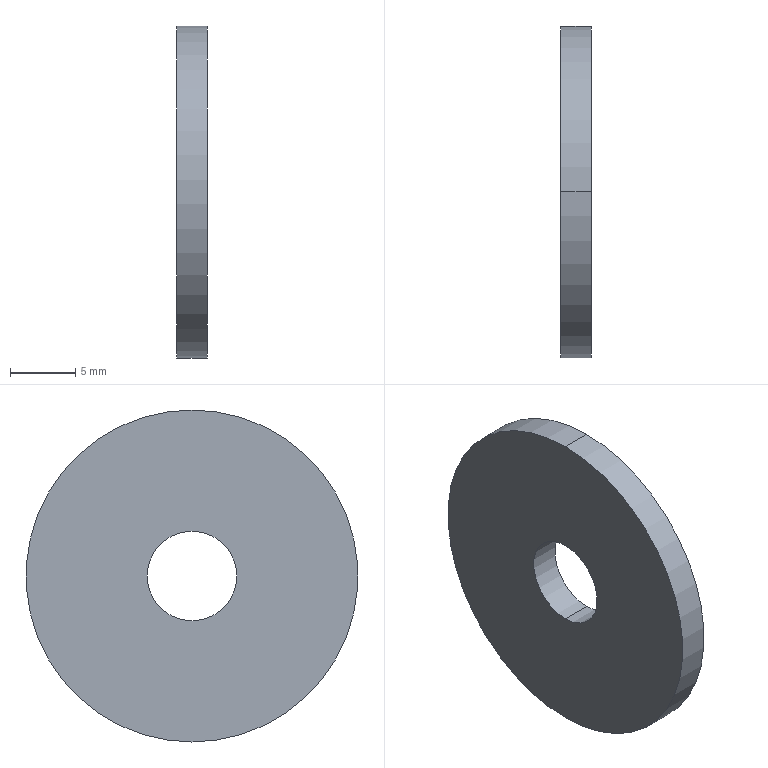Part | STEP file | flat washer wide_am_B18.22M - Plain washer, 6 mm, wide | 1 solid | 6 faces | box 2.3 x 25.4 x 25.4 mm | volume 1080 mm3 | cylinder 4 | plane 2 | commonest cylinder face diameters 6.87 x2 25.4 x2
STEP:
#1=CARTESIAN_POINT('',(0.,0.,0.));
#2=DIRECTION('',(0.,0.,1.));
#3=DIRECTION('',(1.,0.,0.));
#4=AXIS2_PLACEMENT_3D('',#1,#2,#3);
#5=CARTESIAN_POINT('',(0.,0.,12.7));
#6=VERTEX_POINT('',#5);
#7=CARTESIAN_POINT('',(0.,0.,-12.7));
#8=VERTEX_POINT('',#7);
#9=CARTESIAN_POINT('',(0.,0.,0.));
#10=DIRECTION('',(-1.,0.,0.));
#11=DIRECTION('',(0.,0.,1.));
#12=AXIS2_PLACEMENT_3D('',#9,#10,#11);
#13=CIRCLE('',#12,12.7);
#14=CARTESIAN_POINT('',(-34.925,0.,0.));
#15=DIRECTION('',(-1.,0.,0.));
#16=DIRECTION('',(0.,0.,1.));
#17=AXIS2_PLACEMENT_3D('',#14,#15,#16);
#18=CYLINDRICAL_SURFACE('',#17,12.7);
#19=CARTESIAN_POINT('',(0.,-34.925));
#20=DIRECTION('',(1.,0.));
#21=VECTOR('',#20,1.);
#22=LINE('',#19,#21);
#23=(GEOMETRIC_REPRESENTATION_CONTEXT(2)PARAMETRIC_REPRESENTATION_CONTEXT()REPRESENTATION_CONTEXT('',''));
#24=DEFINITIONAL_REPRESENTATION('',(#22),#23);
#25=PCURVE('',#18,#24);
#26=CARTESIAN_POINT('',(0.,3.435,0.));
#27=DIRECTION('',(-1.,0.,0.));
#28=DIRECTION('',(0.,0.,1.));
#29=AXIS2_PLACEMENT_3D('',#26,#27,#28);
#30=PLANE('',#29);
#31=CARTESIAN_POINT('',(0.,-3.435));
#32=DIRECTION('',(1.,0.));
#33=AXIS2_PLACEMENT_2D('',#31,#32);
#34=CIRCLE('',#33,12.7);
#35=(GEOMETRIC_REPRESENTATION_CONTEXT(2)PARAMETRIC_REPRESENTATION_CONTEXT()REPRESENTATION_CONTEXT('',''));
#36=DEFINITIONAL_REPRESENTATION('',(#34),#35);
#37=PCURVE('',#30,#36);
#38=SURFACE_CURVE('',#13,(#25,#37),.PCURVE_S1.);
#39=EDGE_CURVE('',#6,#8,#38,.T.);
#40=ORIENTED_EDGE('',*,*,#39,.T.);
#41=CARTESIAN_POINT('',(-2.3,0.,-12.7));
#42=VERTEX_POINT('',#41);
#43=CARTESIAN_POINT('',(-34.925,0.,-12.7));
#44=DIRECTION('',(-1.,0.,0.));
#45=VECTOR('',#44,1.);
#46=LINE('',#43,#45);
#47=CARTESIAN_POINT('',(3.142,0.));
#48=DIRECTION('',(0.,1.));
#49=VECTOR('',#48,1.);
#50=LINE('',#47,#49);
#51=(GEOMETRIC_REPRESENTATION_CONTEXT(2)PARAMETRIC_REPRESENTATION_CONTEXT()REPRESENTATION_CONTEXT('',''));
#52=DEFINITIONAL_REPRESENTATION('',(#50),#51);
#53=PCURVE('',#18,#52);
#54=CARTESIAN_POINT('',(-34.925,0.,0.));
#55=DIRECTION('',(-1.,0.,0.));
#56=DIRECTION('',(0.,0.,1.));
#57=AXIS2_PLACEMENT_3D('',#54,#55,#56);
#58=CYLINDRICAL_SURFACE('',#57,12.7);
#59=CARTESIAN_POINT('',(3.142,0.));
#60=DIRECTION('',(0.,1.));
#61=VECTOR('',#60,1.);
#62=LINE('',#59,#61);
#63=(GEOMETRIC_REPRESENTATION_CONTEXT(2)PARAMETRIC_REPRESENTATION_CONTEXT()REPRESENTATION_CONTEXT('',''));
#64=DEFINITIONAL_REPRESENTATION('',(#62),#63);
#65=PCURVE('',#58,#64);
#66=SURFACE_CURVE('',#46,(#53,#65),.PCURVE_S1.);
#67=EDGE_CURVE('',#8,#42,#66,.T.);
#68=ORIENTED_EDGE('',*,*,#67,.T.);
#69=CARTESIAN_POINT('',(-2.3,0.,12.7));
#70=VERTEX_POINT('',#69);
#71=CARTESIAN_POINT('',(-2.3,0.,0.));
#72=DIRECTION('',(-1.,0.,0.));
#73=DIRECTION('',(0.,0.,1.));
#74=AXIS2_PLACEMENT_3D('',#71,#72,#73);
#75=CIRCLE('',#74,12.7);
#76=CARTESIAN_POINT('',(0.,-32.625));
#77=DIRECTION('',(1.,0.));
#78=VECTOR('',#77,1.);
#79=LINE('',#76,#78);
#80=(GEOMETRIC_REPRESENTATION_CONTEXT(2)PARAMETRIC_REPRESENTATION_CONTEXT()REPRESENTATION_CONTEXT('',''));
#81=DEFINITIONAL_REPRESENTATION('',(#79),#80);
#82=PCURVE('',#18,#81);
#83=CARTESIAN_POINT('',(-2.3,12.7,0.));
#84=DIRECTION('',(1.,0.,0.));
#85=DIRECTION('',(0.,0.,-1.));
#86=AXIS2_PLACEMENT_3D('',#83,#84,#85);
#87=PLANE('',#86);
#88=CARTESIAN_POINT('',(-12.7,-12.7));
#89=CARTESIAN_POINT('',(-12.7,9.297));
#90=CARTESIAN_POINT('',(6.35,-1.701));
#91=CARTESIAN_POINT('',(25.4,-12.7));
#92=CARTESIAN_POINT('',(6.35,-23.699));
#93=CARTESIAN_POINT('',(-12.7,-34.697));
#94=CARTESIAN_POINT('',(-12.7,-12.7));
#95=(BOUNDED_CURVE()B_SPLINE_CURVE(2,(#88,#89,#90,#91,#92,#93,#94),.UNSPECIFIED.,.T.,.F.)B_SPLINE_CURVE_WITH_KNOTS((1,2,2,2,2,1),(-2.094,0.,2.094,4.189,6.283,8.378),.UNSPECIFIED.)CURVE()GEOMETRIC_REPRESENTATION_ITEM()RATIONAL_B_SPLINE_CURVE((1.,0.5,1.,0.5,1.,0.5,1.))REPRESENTATION_ITEM(''));
#96=(GEOMETRIC_REPRESENTATION_CONTEXT(2)PARAMETRIC_REPRESENTATION_CONTEXT()REPRESENTATION_CONTEXT('',''));
#97=DEFINITIONAL_REPRESENTATION('',(#95),#96);
#98=PCURVE('',#87,#97);
#99=SURFACE_CURVE('',#75,(#82,#98),.PCURVE_S1.);
#100=EDGE_CURVE('',#70,#42,#99,.T.);
#101=ORIENTED_EDGE('',*,*,#100,.F.);
#102=CARTESIAN_POINT('',(-34.925,0.,12.7));
#103=DIRECTION('',(-1.,0.,0.));
#104=VECTOR('',#103,1.);
#105=LINE('',#102,#104);
#106=CARTESIAN_POINT('',(0.,0.));
#107=DIRECTION('',(0.,1.));
#108=VECTOR('',#107,1.);
#109=LINE('',#106,#108);
#110=(GEOMETRIC_REPRESENTATION_CONTEXT(2)PARAMETRIC_REPRESENTATION_CONTEXT()REPRESENTATION_CONTEXT('',''));
#111=DEFINITIONAL_REPRESENTATION('',(#109),#110);
#112=PCURVE('',#18,#111);
#113=CARTESIAN_POINT('',(6.283,0.));
#114=DIRECTION('',(0.,1.));
#115=VECTOR('',#114,1.);
#116=LINE('',#113,#115);
#117=(GEOMETRIC_REPRESENTATION_CONTEXT(2)PARAMETRIC_REPRESENTATION_CONTEXT()REPRESENTATION_CONTEXT('',''));
#118=DEFINITIONAL_REPRESENTATION('',(#116),#117);
#119=PCURVE('',#58,#118);
#120=SURFACE_CURVE('',#105,(#112,#119),.PCURVE_S1.);
#121=EDGE_CURVE('',#6,#70,#120,.T.);
#122=ORIENTED_EDGE('',*,*,#121,.F.);
#123=EDGE_LOOP('',(#40,#68,#101,#122));
#124=FACE_BOUND('',#123,.T.);
#125=ADVANCED_FACE('',(#124),#18,.T.);
#126=CARTESIAN_POINT('',(0.,0.,3.435));
#127=VERTEX_POINT('',#126);
#128=CARTESIAN_POINT('',(-2.3,0.,3.435));
#129=VERTEX_POINT('',#128);
#130=CARTESIAN_POINT('',(-34.925,0.,3.435));
#131=DIRECTION('',(-1.,0.,0.));
#132=VECTOR('',#131,1.);
#133=LINE('',#130,#132);
#134=CARTESIAN_POINT('',(-34.925,0.,0.));
#135=DIRECTION('',(-1.,0.,0.));
#136=DIRECTION('',(0.,0.,1.));
#137=AXIS2_PLACEMENT_3D('',#134,#135,#136);
#138=CYLINDRICAL_SURFACE('',#137,3.435);
#139=CARTESIAN_POINT('',(6.283,0.));
#140=DIRECTION('',(0.,1.));
#141=VECTOR('',#140,1.);
#142=LINE('',#139,#141);
#143=(GEOMETRIC_REPRESENTATION_CONTEXT(2)PARAMETRIC_REPRESENTATION_CONTEXT()REPRESENTATION_CONTEXT('',''));
#144=DEFINITIONAL_REPRESENTATION('',(#142),#143);
#145=PCURVE('',#138,#144);
#146=CARTESIAN_POINT('',(-34.925,0.,0.));
#147=DIRECTION('',(-1.,0.,0.));
#148=DIRECTION('',(0.,0.,1.));
#149=AXIS2_PLACEMENT_3D('',#146,#147,#148);
#150=CYLINDRICAL_SURFACE('',#149,3.435);
#151=CARTESIAN_POINT('',(0.,0.));
#152=DIRECTION('',(0.,1.));
#153=VECTOR('',#152,1.);
#154=LINE('',#151,#153);
#155=(GEOMETRIC_REPRESENTATION_CONTEXT(2)PARAMETRIC_REPRESENTATION_CONTEXT()REPRESENTATION_CONTEXT('',''));
#156=DEFINITIONAL_REPRESENTATION('',(#154),#155);
#157=PCURVE('',#150,#156);
#158=SURFACE_CURVE('',#133,(#145,#157),.PCURVE_S1.);
#159=EDGE_CURVE('',#127,#129,#158,.T.);
#160=ORIENTED_EDGE('',*,*,#159,.T.);
#161=CARTESIAN_POINT('',(-2.3,0.,-3.435));
#162=VERTEX_POINT('',#161);
#163=CARTESIAN_POINT('',(-2.3,0.,0.));
#164=DIRECTION('',(-1.,0.,0.));
#165=DIRECTION('',(0.,0.,1.));
#166=AXIS2_PLACEMENT_3D('',#163,#164,#165);
#167=CIRCLE('',#166,3.435);
#168=CARTESIAN_POINT('',(0.,-32.625));
#169=DIRECTION('',(1.,0.));
#170=VECTOR('',#169,1.);
#171=LINE('',#168,#170);
#172=(GEOMETRIC_REPRESENTATION_CONTEXT(2)PARAMETRIC_REPRESENTATION_CONTEXT()REPRESENTATION_CONTEXT('',''));
#173=DEFINITIONAL_REPRESENTATION('',(#171),#172);
#174=PCURVE('',#138,#173);
#175=CARTESIAN_POINT('',(-3.435,-12.7));
#176=CARTESIAN_POINT('',(-3.435,-6.75));
#177=CARTESIAN_POINT('',(1.718,-9.725));
#178=CARTESIAN_POINT('',(6.87,-12.7));
#179=CARTESIAN_POINT('',(1.718,-15.675));
#180=CARTESIAN_POINT('',(-3.435,-18.65));
#181=CARTESIAN_POINT('',(-3.435,-12.7));
#182=(BOUNDED_CURVE()B_SPLINE_CURVE(2,(#175,#176,#177,#178,#179,#180,#181),.UNSPECIFIED.,.T.,.F.)B_SPLINE_CURVE_WITH_KNOTS((1,2,2,2,2,1),(-2.094,0.,2.094,4.189,6.283,8.378),.UNSPECIFIED.)CURVE()GEOMETRIC_REPRESENTATION_ITEM()RATIONAL_B_SPLINE_CURVE((1.,0.5,1.,0.5,1.,0.5,1.))REPRESENTATION_ITEM(''));
#183=(GEOMETRIC_REPRESENTATION_CONTEXT(2)PARAMETRIC_REPRESENTATION_CONTEXT()REPRESENTATION_CONTEXT('',''));
#184=DEFINITIONAL_REPRESENTATION('',(#182),#183);
#185=PCURVE('',#87,#184);
#186=SURFACE_CURVE('',#167,(#174,#185),.PCURVE_S1.);
#187=EDGE_CURVE('',#162,#129,#186,.T.);
#188=ORIENTED_EDGE('',*,*,#187,.F.);
#189=CARTESIAN_POINT('',(0.,0.,-3.435));
#190=VERTEX_POINT('',#189);
#191=CARTESIAN_POINT('',(-34.925,0.,-3.435));
#192=DIRECTION('',(-1.,0.,0.));
#193=VECTOR('',#192,1.);
#194=LINE('',#191,#193);
#195=CARTESIAN_POINT('',(3.142,0.));
#196=DIRECTION('',(0.,1.));
#197=VECTOR('',#196,1.);
#198=LINE('',#195,#197);
#199=(GEOMETRIC_REPRESENTATION_CONTEXT(2)PARAMETRIC_REPRESENTATION_CONTEXT()REPRESENTATION_CONTEXT('',''));
#200=DEFINITIONAL_REPRESENTATION('',(#198),#199);
#201=PCURVE('',#138,#200);
#202=CARTESIAN_POINT('',(3.142,0.));
#203=DIRECTION('',(0.,1.));
#204=VECTOR('',#203,1.);
#205=LINE('',#202,#204);
#206=(GEOMETRIC_REPRESENTATION_CONTEXT(2)PARAMETRIC_REPRESENTATION_CONTEXT()REPRESENTATION_CONTEXT('',''));
#207=DEFINITIONAL_REPRESENTATION('',(#205),#206);
#208=PCURVE('',#150,#207);
#209=SURFACE_CURVE('',#194,(#201,#208),.PCURVE_S1.);
#210=EDGE_CURVE('',#190,#162,#209,.T.);
#211=ORIENTED_EDGE('',*,*,#210,.F.);
#212=CARTESIAN_POINT('',(0.,0.,0.));
#213=DIRECTION('',(-1.,0.,0.));
#214=DIRECTION('',(0.,0.,1.));
#215=AXIS2_PLACEMENT_3D('',#212,#213,#214);
#216=CIRCLE('',#215,3.435);
#217=CARTESIAN_POINT('',(0.,-34.925));
#218=DIRECTION('',(1.,0.));
#219=VECTOR('',#218,1.);
#220=LINE('',#217,#219);
#221=(GEOMETRIC_REPRESENTATION_CONTEXT(2)PARAMETRIC_REPRESENTATION_CONTEXT()REPRESENTATION_CONTEXT('',''));
#222=DEFINITIONAL_REPRESENTATION('',(#220),#221);
#223=PCURVE('',#138,#222);
#224=CARTESIAN_POINT('',(0.,-3.435));
#225=DIRECTION('',(1.,0.));
#226=AXIS2_PLACEMENT_2D('',#224,#225);
#227=CIRCLE('',#226,3.435);
#228=(GEOMETRIC_REPRESENTATION_CONTEXT(2)PARAMETRIC_REPRESENTATION_CONTEXT()REPRESENTATION_CONTEXT('',''));
#229=DEFINITIONAL_REPRESENTATION('',(#227),#228);
#230=PCURVE('',#30,#229);
#231=SURFACE_CURVE('',#216,(#223,#230),.PCURVE_S1.);
#232=EDGE_CURVE('',#190,#127,#231,.T.);
#233=ORIENTED_EDGE('',*,*,#232,.T.);
#234=EDGE_LOOP('',(#160,#188,#211,#233));
#235=FACE_BOUND('',#234,.F.);
#236=ADVANCED_FACE('',(#235),#138,.F.);
#237=CARTESIAN_POINT('',(-2.3,0.,0.));
#238=DIRECTION('',(-1.,0.,0.));
#239=DIRECTION('',(0.,0.,1.));
#240=AXIS2_PLACEMENT_3D('',#237,#238,#239);
#241=CIRCLE('',#240,3.435);
#242=CARTESIAN_POINT('',(0.,-32.625));
#243=DIRECTION('',(1.,0.));
#244=VECTOR('',#243,1.);
#245=LINE('',#242,#244);
#246=(GEOMETRIC_REPRESENTATION_CONTEXT(2)PARAMETRIC_REPRESENTATION_CONTEXT()REPRESENTATION_CONTEXT('',''));
#247=DEFINITIONAL_REPRESENTATION('',(#245),#246);
#248=PCURVE('',#150,#247);
#249=CARTESIAN_POINT('',(-3.435,-12.7));
#250=CARTESIAN_POINT('',(-3.435,-6.75));
#251=CARTESIAN_POINT('',(1.718,-9.725));
#252=CARTESIAN_POINT('',(6.87,-12.7));
#253=CARTESIAN_POINT('',(1.718,-15.675));
#254=CARTESIAN_POINT('',(-3.435,-18.65));
#255=CARTESIAN_POINT('',(-3.435,-12.7));
#256=(BOUNDED_CURVE()B_SPLINE_CURVE(2,(#249,#250,#251,#252,#253,#254,#255),.UNSPECIFIED.,.T.,.F.)B_SPLINE_CURVE_WITH_KNOTS((1,2,2,2,2,1),(-2.094,0.,2.094,4.189,6.283,8.378),.UNSPECIFIED.)CURVE()GEOMETRIC_REPRESENTATION_ITEM()RATIONAL_B_SPLINE_CURVE((1.,0.5,1.,0.5,1.,0.5,1.))REPRESENTATION_ITEM(''));
#257=(GEOMETRIC_REPRESENTATION_CONTEXT(2)PARAMETRIC_REPRESENTATION_CONTEXT()REPRESENTATION_CONTEXT('',''));
#258=DEFINITIONAL_REPRESENTATION('',(#256),#257);
#259=PCURVE('',#87,#258);
#260=SURFACE_CURVE('',#241,(#248,#259),.PCURVE_S1.);
#261=EDGE_CURVE('',#129,#162,#260,.T.);
#262=ORIENTED_EDGE('',*,*,#261,.F.);
#263=ORIENTED_EDGE('',*,*,#159,.F.);
#264=CARTESIAN_POINT('',(0.,0.,0.));
#265=DIRECTION('',(-1.,0.,0.));
#266=DIRECTION('',(0.,0.,1.));
#267=AXIS2_PLACEMENT_3D('',#264,#265,#266);
#268=CIRCLE('',#267,3.435);
#269=CARTESIAN_POINT('',(0.,-34.925));
#270=DIRECTION('',(1.,0.));
#271=VECTOR('',#270,1.);
#272=LINE('',#269,#271);
#273=(GEOMETRIC_REPRESENTATION_CONTEXT(2)PARAMETRIC_REPRESENTATION_CONTEXT()REPRESENTATION_CONTEXT('',''));
#274=DEFINITIONAL_REPRESENTATION('',(#272),#273);
#275=PCURVE('',#150,#274);
#276=CARTESIAN_POINT('',(0.,-3.435));
#277=DIRECTION('',(1.,0.));
#278=AXIS2_PLACEMENT_2D('',#276,#277);
#279=CIRCLE('',#278,3.435);
#280=(GEOMETRIC_REPRESENTATION_CONTEXT(2)PARAMETRIC_REPRESENTATION_CONTEXT()REPRESENTATION_CONTEXT('',''));
#281=DEFINITIONAL_REPRESENTATION('',(#279),#280);
#282=PCURVE('',#30,#281);
#283=SURFACE_CURVE('',#268,(#275,#282),.PCURVE_S1.);
#284=EDGE_CURVE('',#127,#190,#283,.T.);
#285=ORIENTED_EDGE('',*,*,#284,.T.);
#286=ORIENTED_EDGE('',*,*,#210,.T.);
#287=EDGE_LOOP('',(#262,#263,#285,#286));
#288=FACE_BOUND('',#287,.F.);
#289=ADVANCED_FACE('',(#288),#150,.F.);
#290=ORIENTED_EDGE('',*,*,#39,.F.);
#291=CARTESIAN_POINT('',(0.,0.,0.));
#292=DIRECTION('',(-1.,0.,0.));
#293=DIRECTION('',(0.,0.,1.));
#294=AXIS2_PLACEMENT_3D('',#291,#292,#293);
#295=CIRCLE('',#294,12.7);
#296=CARTESIAN_POINT('',(0.,-3.435));
#297=DIRECTION('',(1.,0.));
#298=AXIS2_PLACEMENT_2D('',#296,#297);
#299=CIRCLE('',#298,12.7);
#300=(GEOMETRIC_REPRESENTATION_CONTEXT(2)PARAMETRIC_REPRESENTATION_CONTEXT()REPRESENTATION_CONTEXT('',''));
#301=DEFINITIONAL_REPRESENTATION('',(#299),#300);
#302=PCURVE('',#30,#301);
#303=CARTESIAN_POINT('',(0.,-34.925));
#304=DIRECTION('',(1.,0.));
#305=VECTOR('',#304,1.);
#306=LINE('',#303,#305);
#307=(GEOMETRIC_REPRESENTATION_CONTEXT(2)PARAMETRIC_REPRESENTATION_CONTEXT()REPRESENTATION_CONTEXT('',''));
#308=DEFINITIONAL_REPRESENTATION('',(#306),#307);
#309=PCURVE('',#58,#308);
#310=SURFACE_CURVE('',#295,(#302,#309),.PCURVE_S1.);
#311=EDGE_CURVE('',#8,#6,#310,.T.);
#312=ORIENTED_EDGE('',*,*,#311,.F.);
#313=EDGE_LOOP('',(#290,#312));
#314=FACE_BOUND('',#313,.T.);
#315=ORIENTED_EDGE('',*,*,#284,.T.);
#316=ORIENTED_EDGE('',*,*,#232,.T.);
#317=EDGE_LOOP('',(#315,#316));
#318=FACE_BOUND('',#317,.T.);
#319=ADVANCED_FACE('',(#314,#318),#30,.F.);
#320=ORIENTED_EDGE('',*,*,#67,.F.);
#321=ORIENTED_EDGE('',*,*,#311,.T.);
#322=ORIENTED_EDGE('',*,*,#121,.T.);
#323=CARTESIAN_POINT('',(-2.3,0.,0.));
#324=DIRECTION('',(-1.,0.,0.));
#325=DIRECTION('',(0.,0.,1.));
#326=AXIS2_PLACEMENT_3D('',#323,#324,#325);
#327=CIRCLE('',#326,12.7);
#328=CARTESIAN_POINT('',(0.,-32.625));
#329=DIRECTION('',(1.,0.));
#330=VECTOR('',#329,1.);
#331=LINE('',#328,#330);
#332=(GEOMETRIC_REPRESENTATION_CONTEXT(2)PARAMETRIC_REPRESENTATION_CONTEXT()REPRESENTATION_CONTEXT('',''));
#333=DEFINITIONAL_REPRESENTATION('',(#331),#332);
#334=PCURVE('',#58,#333);
#335=CARTESIAN_POINT('',(-12.7,-12.7));
#336=CARTESIAN_POINT('',(-12.7,9.297));
#337=CARTESIAN_POINT('',(6.35,-1.701));
#338=CARTESIAN_POINT('',(25.4,-12.7));
#339=CARTESIAN_POINT('',(6.35,-23.699));
#340=CARTESIAN_POINT('',(-12.7,-34.697));
#341=CARTESIAN_POINT('',(-12.7,-12.7));
#342=(BOUNDED_CURVE()B_SPLINE_CURVE(2,(#335,#336,#337,#338,#339,#340,#341),.UNSPECIFIED.,.T.,.F.)B_SPLINE_CURVE_WITH_KNOTS((1,2,2,2,2,1),(-2.094,0.,2.094,4.189,6.283,8.378),.UNSPECIFIED.)CURVE()GEOMETRIC_REPRESENTATION_ITEM()RATIONAL_B_SPLINE_CURVE((1.,0.5,1.,0.5,1.,0.5,1.))REPRESENTATION_ITEM(''));
#343=(GEOMETRIC_REPRESENTATION_CONTEXT(2)PARAMETRIC_REPRESENTATION_CONTEXT()REPRESENTATION_CONTEXT('',''));
#344=DEFINITIONAL_REPRESENTATION('',(#342),#343);
#345=PCURVE('',#87,#344);
#346=SURFACE_CURVE('',#327,(#334,#345),.PCURVE_S1.);
#347=EDGE_CURVE('',#42,#70,#346,.T.);
#348=ORIENTED_EDGE('',*,*,#347,.F.);
#349=EDGE_LOOP('',(#320,#321,#322,#348));
#350=FACE_BOUND('',#349,.T.);
#351=ADVANCED_FACE('',(#350),#58,.T.);
#352=ORIENTED_EDGE('',*,*,#261,.F.);
#353=ORIENTED_EDGE('',*,*,#187,.F.);
#354=EDGE_LOOP('',(#352,#353));
#355=FACE_BOUND('',#354,.T.);
#356=ORIENTED_EDGE('',*,*,#100,.T.);
#357=ORIENTED_EDGE('',*,*,#347,.T.);
#358=EDGE_LOOP('',(#356,#357));
#359=FACE_BOUND('',#358,.T.);
#360=ADVANCED_FACE('',(#355,#359),#87,.F.);
#361=CLOSED_SHELL('',(#125,#236,#289,#319,#351,#360));
#362=MANIFOLD_SOLID_BREP('',#361);
#363=(LENGTH_UNIT()NAMED_UNIT(*)SI_UNIT(.MILLI.,.METRE.));
#364=UNCERTAINTY_MEASURE_WITH_UNIT(LENGTH_MEASURE(0.0000001),#363,'','');
#365=(NAMED_UNIT(*)PLANE_ANGLE_UNIT()SI_UNIT($,.RADIAN.));
#366=(NAMED_UNIT(*)SI_UNIT($,.STERADIAN.)SOLID_ANGLE_UNIT());
#367=(GEOMETRIC_REPRESENTATION_CONTEXT(3)GLOBAL_UNCERTAINTY_ASSIGNED_CONTEXT((#364))GLOBAL_UNIT_ASSIGNED_CONTEXT((#363,#365,#366))REPRESENTATION_CONTEXT('',''));
#368=ADVANCED_BREP_SHAPE_REPRESENTATION('',(#4,#362),#367);